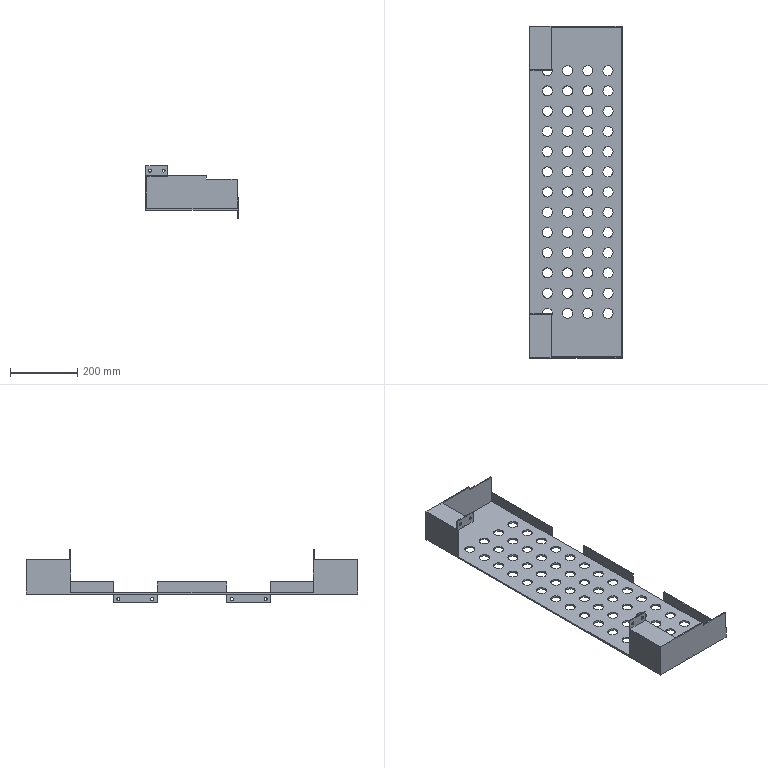Part | NX | features DATUM_CSYS 13, EXTRUDE 12, SKETCH 12, OFFSET_REGION 2 | 1 solid | 110 faces | box 274 x 985 x 157 mm | volume 1535360 mm3 | cylinder 60 | plane 50 | commonest cylinder face diameters 30 x52 9 x8